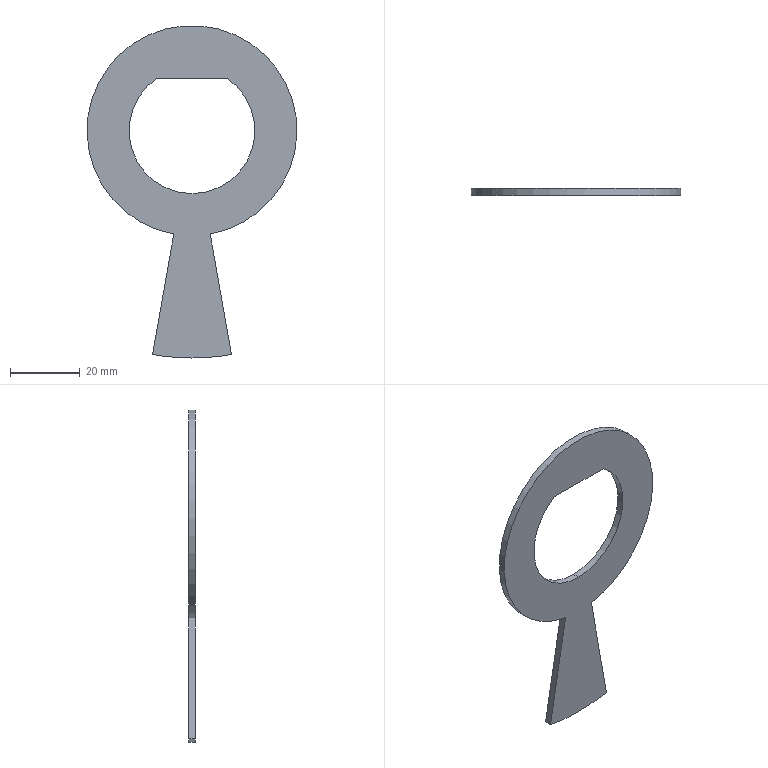Part | STEP file | 10-09 sensor plate | 1 solid | 10 faces | box 60 x 2 x 95 mm | volume 4861 mm3 | cylinder 5 | plane 5 | commonest cylinder face diameters 36 x2 130 x2 60 x1
STEP:
#1=CARTESIAN_POINT('',(9.95,2.,15.));
#2=VERTEX_POINT('',#1);
#3=CARTESIAN_POINT('',(0.,2.,-18.));
#4=VERTEX_POINT('',#3);
#5=CARTESIAN_POINT('',(0.,2.,0.));
#6=DIRECTION('',(0.,1.,0.));
#7=DIRECTION('',(0.,0.,1.));
#8=AXIS2_PLACEMENT_3D('',#5,#6,#7);
#9=CIRCLE('',#8,18.);
#10=EDGE_CURVE('',#2,#4,#9,.T.);
#11=ORIENTED_EDGE('',*,*,#10,.T.);
#12=CARTESIAN_POINT('',(0.,0.,-18.));
#13=VERTEX_POINT('',#12);
#14=CARTESIAN_POINT('',(0.,2.,-18.));
#15=DIRECTION('',(0.,-1.,0.));
#16=VECTOR('',#15,1000.);
#17=LINE('',#14,#16);
#18=EDGE_CURVE('',#4,#13,#17,.T.);
#19=ORIENTED_EDGE('',*,*,#18,.T.);
#20=CARTESIAN_POINT('',(9.95,0.,15.));
#21=VERTEX_POINT('',#20);
#22=CARTESIAN_POINT('',(0.,0.,0.));
#23=DIRECTION('',(0.,1.,0.));
#24=DIRECTION('',(0.,0.,1.));
#25=AXIS2_PLACEMENT_3D('',#22,#23,#24);
#26=CIRCLE('',#25,18.);
#27=EDGE_CURVE('',#21,#13,#26,.T.);
#28=ORIENTED_EDGE('',*,*,#27,.F.);
#29=CARTESIAN_POINT('',(9.95,2.,15.));
#30=DIRECTION('',(0.,-1.,0.));
#31=VECTOR('',#30,1000.);
#32=LINE('',#29,#31);
#33=EDGE_CURVE('',#2,#21,#32,.T.);
#34=ORIENTED_EDGE('',*,*,#33,.F.);
#35=EDGE_LOOP('',(#11,#19,#28,#34));
#36=FACE_OUTER_BOUND('',#35,.T.);
#37=CARTESIAN_POINT('',(0.,2.,0.));
#38=DIRECTION('',(0.,-1.,0.));
#39=DIRECTION('',(0.,0.,-1.));
#40=AXIS2_PLACEMENT_3D('',#37,#38,#39);
#41=CYLINDRICAL_SURFACE('',#40,18.);
#42=ADVANCED_FACE('',(#36),#41,.F.);
#43=CARTESIAN_POINT('',(0.,2.,-65.));
#44=VERTEX_POINT('',#43);
#45=CARTESIAN_POINT('',(-11.287,2.,-64.013));
#46=VERTEX_POINT('',#45);
#47=CARTESIAN_POINT('',(0.,2.,0.));
#48=DIRECTION('',(0.,1.,0.));
#49=DIRECTION('',(0.,0.,1.));
#50=AXIS2_PLACEMENT_3D('',#47,#48,#49);
#51=CIRCLE('',#50,65.);
#52=EDGE_CURVE('',#44,#46,#51,.T.);
#53=ORIENTED_EDGE('',*,*,#52,.F.);
#54=CARTESIAN_POINT('',(0.,0.,-65.));
#55=VERTEX_POINT('',#54);
#56=CARTESIAN_POINT('',(0.,2.,-65.));
#57=DIRECTION('',(0.,-1.,0.));
#58=VECTOR('',#57,1000.);
#59=LINE('',#56,#58);
#60=EDGE_CURVE('',#44,#55,#59,.T.);
#61=ORIENTED_EDGE('',*,*,#60,.T.);
#62=CARTESIAN_POINT('',(-11.287,0.,-64.013));
#63=VERTEX_POINT('',#62);
#64=CARTESIAN_POINT('',(0.,0.,0.));
#65=DIRECTION('',(0.,1.,0.));
#66=DIRECTION('',(0.,0.,1.));
#67=AXIS2_PLACEMENT_3D('',#64,#65,#66);
#68=CIRCLE('',#67,65.);
#69=EDGE_CURVE('',#55,#63,#68,.T.);
#70=ORIENTED_EDGE('',*,*,#69,.T.);
#71=CARTESIAN_POINT('',(-11.287,2.,-64.013));
#72=DIRECTION('',(0.,-1.,0.));
#73=VECTOR('',#72,1000.);
#74=LINE('',#71,#73);
#75=EDGE_CURVE('',#46,#63,#74,.T.);
#76=ORIENTED_EDGE('',*,*,#75,.F.);
#77=EDGE_LOOP('',(#53,#61,#70,#76));
#78=FACE_OUTER_BOUND('',#77,.T.);
#79=CARTESIAN_POINT('',(0.,2.,0.));
#80=DIRECTION('',(0.,-1.,0.));
#81=DIRECTION('',(0.,0.,-1.));
#82=AXIS2_PLACEMENT_3D('',#79,#80,#81);
#83=CYLINDRICAL_SURFACE('',#82,65.);
#84=ADVANCED_FACE('',(#78),#83,.T.);
#85=CARTESIAN_POINT('',(11.287,2.,-64.013));
#86=VERTEX_POINT('',#85);
#87=CARTESIAN_POINT('',(0.,2.,0.));
#88=DIRECTION('',(0.,1.,0.));
#89=DIRECTION('',(0.,0.,1.));
#90=AXIS2_PLACEMENT_3D('',#87,#88,#89);
#91=CIRCLE('',#90,65.);
#92=EDGE_CURVE('',#86,#44,#91,.T.);
#93=ORIENTED_EDGE('',*,*,#92,.T.);
#94=ORIENTED_EDGE('',*,*,#52,.T.);
#95=CARTESIAN_POINT('',(-5.209,2.,-29.544));
#96=VERTEX_POINT('',#95);
#97=CARTESIAN_POINT('',(-5.209,2.,-29.544));
#98=DIRECTION('',(0.1736,0.,0.9848));
#99=VECTOR('',#98,1000.);
#100=LINE('',#97,#99);
#101=EDGE_CURVE('',#46,#96,#100,.T.);
#102=ORIENTED_EDGE('',*,*,#101,.T.);
#103=CARTESIAN_POINT('',(5.209,2.,-29.544));
#104=VERTEX_POINT('',#103);
#105=CARTESIAN_POINT('',(0.,2.,0.));
#106=DIRECTION('',(0.,1.,0.));
#107=DIRECTION('',(0.,0.,1.));
#108=AXIS2_PLACEMENT_3D('',#105,#106,#107);
#109=CIRCLE('',#108,30.);
#110=EDGE_CURVE('',#96,#104,#109,.T.);
#111=ORIENTED_EDGE('',*,*,#110,.T.);
#112=CARTESIAN_POINT('',(5.209,2.,-29.544));
#113=DIRECTION('',(0.1736,0.,-0.9848));
#114=VECTOR('',#113,1000.);
#115=LINE('',#112,#114);
#116=EDGE_CURVE('',#104,#86,#115,.T.);
#117=ORIENTED_EDGE('',*,*,#116,.T.);
#118=EDGE_LOOP('',(#93,#94,#102,#111,#117));
#119=FACE_OUTER_BOUND('',#118,.T.);
#120=CARTESIAN_POINT('',(-9.95,2.,15.));
#121=VERTEX_POINT('',#120);
#122=CARTESIAN_POINT('',(-9.95,2.,15.));
#123=DIRECTION('',(1.,0.,0.));
#124=VECTOR('',#123,1000.);
#125=LINE('',#122,#124);
#126=EDGE_CURVE('',#121,#2,#125,.T.);
#127=ORIENTED_EDGE('',*,*,#126,.F.);
#128=CARTESIAN_POINT('',(0.,2.,0.));
#129=DIRECTION('',(0.,1.,0.));
#130=DIRECTION('',(0.,0.,1.));
#131=AXIS2_PLACEMENT_3D('',#128,#129,#130);
#132=CIRCLE('',#131,18.);
#133=EDGE_CURVE('',#4,#121,#132,.T.);
#134=ORIENTED_EDGE('',*,*,#133,.F.);
#135=ORIENTED_EDGE('',*,*,#10,.F.);
#136=EDGE_LOOP('',(#127,#134,#135));
#137=FACE_BOUND('',#136,.T.);
#138=CARTESIAN_POINT('',(0.,2.,0.));
#139=DIRECTION('',(0.,1.,0.));
#140=DIRECTION('',(0.,0.,1.));
#141=AXIS2_PLACEMENT_3D('',#138,#139,#140);
#142=PLANE('',#141);
#143=ADVANCED_FACE('',(#119,#137),#142,.T.);
#144=CARTESIAN_POINT('',(11.287,0.,-64.013));
#145=VERTEX_POINT('',#144);
#146=CARTESIAN_POINT('',(0.,0.,0.));
#147=DIRECTION('',(0.,1.,0.));
#148=DIRECTION('',(0.,0.,1.));
#149=AXIS2_PLACEMENT_3D('',#146,#147,#148);
#150=CIRCLE('',#149,65.);
#151=EDGE_CURVE('',#145,#55,#150,.T.);
#152=ORIENTED_EDGE('',*,*,#151,.F.);
#153=CARTESIAN_POINT('',(5.209,0.,-29.544));
#154=VERTEX_POINT('',#153);
#155=CARTESIAN_POINT('',(5.209,0.,-29.544));
#156=DIRECTION('',(0.1736,0.,-0.9848));
#157=VECTOR('',#156,1000.);
#158=LINE('',#155,#157);
#159=EDGE_CURVE('',#154,#145,#158,.T.);
#160=ORIENTED_EDGE('',*,*,#159,.F.);
#161=CARTESIAN_POINT('',(-5.209,0.,-29.544));
#162=VERTEX_POINT('',#161);
#163=CARTESIAN_POINT('',(0.,0.,0.));
#164=DIRECTION('',(0.,1.,0.));
#165=DIRECTION('',(0.,0.,1.));
#166=AXIS2_PLACEMENT_3D('',#163,#164,#165);
#167=CIRCLE('',#166,30.);
#168=EDGE_CURVE('',#162,#154,#167,.T.);
#169=ORIENTED_EDGE('',*,*,#168,.F.);
#170=CARTESIAN_POINT('',(-5.209,0.,-29.544));
#171=DIRECTION('',(0.1736,0.,0.9848));
#172=VECTOR('',#171,1000.);
#173=LINE('',#170,#172);
#174=EDGE_CURVE('',#63,#162,#173,.T.);
#175=ORIENTED_EDGE('',*,*,#174,.F.);
#176=ORIENTED_EDGE('',*,*,#69,.F.);
#177=EDGE_LOOP('',(#152,#160,#169,#175,#176));
#178=FACE_OUTER_BOUND('',#177,.T.);
#179=ORIENTED_EDGE('',*,*,#27,.T.);
#180=CARTESIAN_POINT('',(-9.95,0.,15.));
#181=VERTEX_POINT('',#180);
#182=CARTESIAN_POINT('',(0.,0.,0.));
#183=DIRECTION('',(0.,1.,0.));
#184=DIRECTION('',(0.,0.,1.));
#185=AXIS2_PLACEMENT_3D('',#182,#183,#184);
#186=CIRCLE('',#185,18.);
#187=EDGE_CURVE('',#13,#181,#186,.T.);
#188=ORIENTED_EDGE('',*,*,#187,.T.);
#189=CARTESIAN_POINT('',(-9.95,0.,15.));
#190=DIRECTION('',(1.,0.,0.));
#191=VECTOR('',#190,1000.);
#192=LINE('',#189,#191);
#193=EDGE_CURVE('',#181,#21,#192,.T.);
#194=ORIENTED_EDGE('',*,*,#193,.T.);
#195=EDGE_LOOP('',(#179,#188,#194));
#196=FACE_BOUND('',#195,.T.);
#197=CARTESIAN_POINT('',(0.,0.,0.));
#198=DIRECTION('',(0.,1.,0.));
#199=DIRECTION('',(0.,0.,1.));
#200=AXIS2_PLACEMENT_3D('',#197,#198,#199);
#201=PLANE('',#200);
#202=ADVANCED_FACE('',(#178,#196),#201,.F.);
#203=ORIENTED_EDGE('',*,*,#60,.F.);
#204=ORIENTED_EDGE('',*,*,#92,.F.);
#205=CARTESIAN_POINT('',(11.287,2.,-64.013));
#206=DIRECTION('',(0.,-1.,0.));
#207=VECTOR('',#206,1000.);
#208=LINE('',#205,#207);
#209=EDGE_CURVE('',#86,#145,#208,.T.);
#210=ORIENTED_EDGE('',*,*,#209,.T.);
#211=ORIENTED_EDGE('',*,*,#151,.T.);
#212=EDGE_LOOP('',(#203,#204,#210,#211));
#213=FACE_OUTER_BOUND('',#212,.T.);
#214=CARTESIAN_POINT('',(0.,2.,0.));
#215=DIRECTION('',(0.,-1.,0.));
#216=DIRECTION('',(0.,0.,-1.));
#217=AXIS2_PLACEMENT_3D('',#214,#215,#216);
#218=CYLINDRICAL_SURFACE('',#217,65.);
#219=ADVANCED_FACE('',(#213),#218,.T.);
#220=ORIENTED_EDGE('',*,*,#174,.T.);
#221=CARTESIAN_POINT('',(-5.209,2.,-29.544));
#222=DIRECTION('',(0.,-1.,0.));
#223=VECTOR('',#222,1000.);
#224=LINE('',#221,#223);
#225=EDGE_CURVE('',#96,#162,#224,.T.);
#226=ORIENTED_EDGE('',*,*,#225,.F.);
#227=ORIENTED_EDGE('',*,*,#101,.F.);
#228=ORIENTED_EDGE('',*,*,#75,.T.);
#229=EDGE_LOOP('',(#220,#226,#227,#228));
#230=FACE_OUTER_BOUND('',#229,.T.);
#231=CARTESIAN_POINT('',(-5.209,2.,-29.544));
#232=DIRECTION('',(0.9848,0.,-0.1736));
#233=DIRECTION('',(-0.1736,0.,-0.9848));
#234=AXIS2_PLACEMENT_3D('',#231,#232,#233);
#235=PLANE('',#234);
#236=ADVANCED_FACE('',(#230),#235,.F.);
#237=ORIENTED_EDGE('',*,*,#168,.T.);
#238=CARTESIAN_POINT('',(5.209,2.,-29.544));
#239=DIRECTION('',(0.,-1.,0.));
#240=VECTOR('',#239,1000.);
#241=LINE('',#238,#240);
#242=EDGE_CURVE('',#104,#154,#241,.T.);
#243=ORIENTED_EDGE('',*,*,#242,.F.);
#244=ORIENTED_EDGE('',*,*,#110,.F.);
#245=ORIENTED_EDGE('',*,*,#225,.T.);
#246=EDGE_LOOP('',(#237,#243,#244,#245));
#247=FACE_OUTER_BOUND('',#246,.T.);
#248=CARTESIAN_POINT('',(0.,2.,0.));
#249=DIRECTION('',(0.,-1.,0.));
#250=DIRECTION('',(0.,0.,-1.));
#251=AXIS2_PLACEMENT_3D('',#248,#249,#250);
#252=CYLINDRICAL_SURFACE('',#251,30.);
#253=ADVANCED_FACE('',(#247),#252,.T.);
#254=ORIENTED_EDGE('',*,*,#159,.T.);
#255=ORIENTED_EDGE('',*,*,#209,.F.);
#256=ORIENTED_EDGE('',*,*,#116,.F.);
#257=ORIENTED_EDGE('',*,*,#242,.T.);
#258=EDGE_LOOP('',(#254,#255,#256,#257));
#259=FACE_OUTER_BOUND('',#258,.T.);
#260=CARTESIAN_POINT('',(5.209,2.,-29.544));
#261=DIRECTION('',(-0.9848,0.,-0.1736));
#262=DIRECTION('',(-0.1736,0.,0.9848));
#263=AXIS2_PLACEMENT_3D('',#260,#261,#262);
#264=PLANE('',#263);
#265=ADVANCED_FACE('',(#259),#264,.F.);
#266=ORIENTED_EDGE('',*,*,#18,.F.);
#267=ORIENTED_EDGE('',*,*,#133,.T.);
#268=CARTESIAN_POINT('',(-9.95,2.,15.));
#269=DIRECTION('',(0.,-1.,0.));
#270=VECTOR('',#269,1000.);
#271=LINE('',#268,#270);
#272=EDGE_CURVE('',#121,#181,#271,.T.);
#273=ORIENTED_EDGE('',*,*,#272,.T.);
#274=ORIENTED_EDGE('',*,*,#187,.F.);
#275=EDGE_LOOP('',(#266,#267,#273,#274));
#276=FACE_OUTER_BOUND('',#275,.T.);
#277=CARTESIAN_POINT('',(0.,2.,0.));
#278=DIRECTION('',(0.,-1.,0.));
#279=DIRECTION('',(0.,0.,-1.));
#280=AXIS2_PLACEMENT_3D('',#277,#278,#279);
#281=CYLINDRICAL_SURFACE('',#280,18.);
#282=ADVANCED_FACE('',(#276),#281,.F.);
#283=ORIENTED_EDGE('',*,*,#193,.F.);
#284=ORIENTED_EDGE('',*,*,#272,.F.);
#285=ORIENTED_EDGE('',*,*,#126,.T.);
#286=ORIENTED_EDGE('',*,*,#33,.T.);
#287=EDGE_LOOP('',(#283,#284,#285,#286));
#288=FACE_OUTER_BOUND('',#287,.T.);
#289=CARTESIAN_POINT('',(-9.95,2.,15.));
#290=DIRECTION('',(0.,0.,-1.));
#291=DIRECTION('',(-1.,0.,0.));
#292=AXIS2_PLACEMENT_3D('',#289,#290,#291);
#293=PLANE('',#292);
#294=ADVANCED_FACE('',(#288),#293,.T.);
#295=CLOSED_SHELL('',(#42,#84,#143,#202,#219,#236,#253,#265,#282,#294));
#296=MANIFOLD_SOLID_BREP('',#295);
#297=CARTESIAN_POINT('',(0.,0.,0.));
#298=DIRECTION('',(0.,0.,1.));
#299=DIRECTION('',(1.,0.,0.));
#300=AXIS2_PLACEMENT_3D('',#297,#298,#299);
#301=(LENGTH_UNIT()NAMED_UNIT(*)SI_UNIT(.MILLI.,.METRE.));
#302=UNCERTAINTY_MEASURE_WITH_UNIT(LENGTH_MEASURE(0.00001),#301,'','');
#303=(NAMED_UNIT(*)PLANE_ANGLE_UNIT()SI_UNIT($,.RADIAN.));
#304=(NAMED_UNIT(*)SI_UNIT($,.STERADIAN.)SOLID_ANGLE_UNIT());
#305=(GEOMETRIC_REPRESENTATION_CONTEXT(3)GLOBAL_UNCERTAINTY_ASSIGNED_CONTEXT((#302))GLOBAL_UNIT_ASSIGNED_CONTEXT((#301,#303,#304))REPRESENTATION_CONTEXT('',''));
#306=ADVANCED_BREP_SHAPE_REPRESENTATION('',(#296,#300),#305);